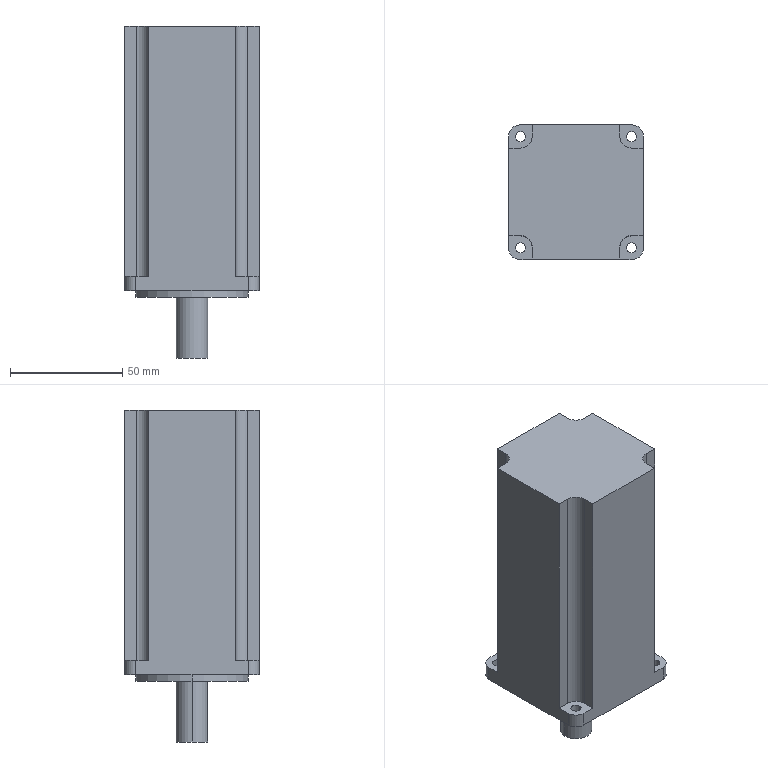Part | SolidWorks | features ICE 3, Extrusion 1 | 1 solid | 40 faces | box 60 x 60 x 148 mm | volume 387738 mm3 | cylinder 20 | plane 20 | commonest cylinder face diameters 4.5 x8 10 x4 10.503 x4 14 x2 50 x2
STEP:
#1=CARTESIAN_POINT('',(-7.,0.,-30.));
#2=VERTEX_POINT('',#1);
#3=CARTESIAN_POINT('',(7.,0.,-30.));
#4=VERTEX_POINT('',#3);
#5=CARTESIAN_POINT('',(0.,0.,-30.));
#6=DIRECTION('',(0.,0.,-1.));
#7=DIRECTION('',(-1.,0.,0.));
#8=AXIS2_PLACEMENT_3D('',#5,#6,#7);
#9=CIRCLE('',#8,7.);
#10=EDGE_CURVE('',#2,#4,#9,.T.);
#11=ORIENTED_EDGE('',*,*,#10,.F.);
#12=CARTESIAN_POINT('',(-7.,0.,-3.));
#13=VERTEX_POINT('',#12);
#14=CARTESIAN_POINT('',(-7.,0.,-30.));
#15=DIRECTION('',(0.,0.,1.));
#16=VECTOR('',#15,1000.);
#17=LINE('',#14,#16);
#18=EDGE_CURVE('',#2,#13,#17,.T.);
#19=ORIENTED_EDGE('',*,*,#18,.T.);
#20=CARTESIAN_POINT('',(7.,0.,-3.));
#21=VERTEX_POINT('',#20);
#22=CARTESIAN_POINT('',(0.,0.,-3.));
#23=DIRECTION('',(0.,0.,-1.));
#24=DIRECTION('',(-1.,0.,0.));
#25=AXIS2_PLACEMENT_3D('',#22,#23,#24);
#26=CIRCLE('',#25,7.);
#27=EDGE_CURVE('',#13,#21,#26,.T.);
#28=ORIENTED_EDGE('',*,*,#27,.T.);
#29=CARTESIAN_POINT('',(7.,0.,-30.));
#30=DIRECTION('',(0.,0.,1.));
#31=VECTOR('',#30,1000.);
#32=LINE('',#29,#31);
#33=EDGE_CURVE('',#4,#21,#32,.T.);
#34=ORIENTED_EDGE('',*,*,#33,.F.);
#35=EDGE_LOOP('',(#11,#19,#28,#34));
#36=FACE_OUTER_BOUND('',#35,.T.);
#37=CARTESIAN_POINT('',(0.,0.,-30.));
#38=DIRECTION('',(0.,0.,1.));
#39=DIRECTION('',(1.,0.,0.));
#40=AXIS2_PLACEMENT_3D('',#37,#38,#39);
#41=CYLINDRICAL_SURFACE('',#40,7.);
#42=ADVANCED_FACE('',(#36),#41,.T.);
#43=CARTESIAN_POINT('',(-25.,0.,-3.));
#44=VERTEX_POINT('',#43);
#45=CARTESIAN_POINT('',(25.,0.,-3.));
#46=VERTEX_POINT('',#45);
#47=CARTESIAN_POINT('',(0.,0.,-3.));
#48=DIRECTION('',(0.,0.,-1.));
#49=DIRECTION('',(-1.,0.,0.));
#50=AXIS2_PLACEMENT_3D('',#47,#48,#49);
#51=CIRCLE('',#50,25.);
#52=EDGE_CURVE('',#44,#46,#51,.T.);
#53=ORIENTED_EDGE('',*,*,#52,.F.);
#54=CARTESIAN_POINT('',(-25.,0.,0.));
#55=VERTEX_POINT('',#54);
#56=CARTESIAN_POINT('',(-25.,0.,-3.));
#57=DIRECTION('',(0.,0.,1.));
#58=VECTOR('',#57,1000.);
#59=LINE('',#56,#58);
#60=EDGE_CURVE('',#44,#55,#59,.T.);
#61=ORIENTED_EDGE('',*,*,#60,.T.);
#62=CARTESIAN_POINT('',(25.,0.,0.));
#63=VERTEX_POINT('',#62);
#64=CARTESIAN_POINT('',(0.,0.,0.));
#65=DIRECTION('',(0.,0.,-1.));
#66=DIRECTION('',(-1.,0.,0.));
#67=AXIS2_PLACEMENT_3D('',#64,#65,#66);
#68=CIRCLE('',#67,25.);
#69=EDGE_CURVE('',#55,#63,#68,.T.);
#70=ORIENTED_EDGE('',*,*,#69,.T.);
#71=CARTESIAN_POINT('',(25.,0.,-3.));
#72=DIRECTION('',(0.,0.,1.));
#73=VECTOR('',#72,1000.);
#74=LINE('',#71,#73);
#75=EDGE_CURVE('',#46,#63,#74,.T.);
#76=ORIENTED_EDGE('',*,*,#75,.F.);
#77=EDGE_LOOP('',(#53,#61,#70,#76));
#78=FACE_OUTER_BOUND('',#77,.T.);
#79=CARTESIAN_POINT('',(0.,0.,-3.));
#80=DIRECTION('',(0.,0.,1.));
#81=DIRECTION('',(1.,0.,0.));
#82=AXIS2_PLACEMENT_3D('',#79,#80,#81);
#83=CYLINDRICAL_SURFACE('',#82,25.);
#84=ADVANCED_FACE('',(#78),#83,.T.);
#85=CARTESIAN_POINT('',(22.499,24.749,6.5));
#86=VERTEX_POINT('',#85);
#87=CARTESIAN_POINT('',(26.999,24.749,6.5));
#88=VERTEX_POINT('',#87);
#89=CARTESIAN_POINT('',(24.749,24.749,6.5));
#90=DIRECTION('',(0.,0.,1.));
#91=DIRECTION('',(1.,0.,0.));
#92=AXIS2_PLACEMENT_3D('',#89,#90,#91);
#93=CIRCLE('',#92,2.25);
#94=EDGE_CURVE('',#86,#88,#93,.T.);
#95=ORIENTED_EDGE('',*,*,#94,.T.);
#96=CARTESIAN_POINT('',(26.999,24.749,0.));
#97=VERTEX_POINT('',#96);
#98=CARTESIAN_POINT('',(26.999,24.749,6.5));
#99=DIRECTION('',(0.,0.,-1.));
#100=VECTOR('',#99,1000.);
#101=LINE('',#98,#100);
#102=EDGE_CURVE('',#88,#97,#101,.T.);
#103=ORIENTED_EDGE('',*,*,#102,.T.);
#104=CARTESIAN_POINT('',(22.499,24.749,0.));
#105=VERTEX_POINT('',#104);
#106=CARTESIAN_POINT('',(24.749,24.749,0.));
#107=DIRECTION('',(0.,0.,1.));
#108=DIRECTION('',(1.,0.,0.));
#109=AXIS2_PLACEMENT_3D('',#106,#107,#108);
#110=CIRCLE('',#109,2.25);
#111=EDGE_CURVE('',#105,#97,#110,.T.);
#112=ORIENTED_EDGE('',*,*,#111,.F.);
#113=CARTESIAN_POINT('',(22.499,24.749,6.5));
#114=DIRECTION('',(0.,0.,-1.));
#115=VECTOR('',#114,1000.);
#116=LINE('',#113,#115);
#117=EDGE_CURVE('',#86,#105,#116,.T.);
#118=ORIENTED_EDGE('',*,*,#117,.F.);
#119=EDGE_LOOP('',(#95,#103,#112,#118));
#120=FACE_OUTER_BOUND('',#119,.T.);
#121=CARTESIAN_POINT('',(24.749,24.749,6.5));
#122=DIRECTION('',(0.,0.,-1.));
#123=DIRECTION('',(-1.,0.,0.));
#124=AXIS2_PLACEMENT_3D('',#121,#122,#123);
#125=CYLINDRICAL_SURFACE('',#124,2.25);
#126=ADVANCED_FACE('',(#120),#125,.F.);
#127=CARTESIAN_POINT('',(22.499,-24.749,6.5));
#128=VERTEX_POINT('',#127);
#129=CARTESIAN_POINT('',(26.999,-24.749,6.5));
#130=VERTEX_POINT('',#129);
#131=CARTESIAN_POINT('',(24.749,-24.749,6.5));
#132=DIRECTION('',(0.,0.,1.));
#133=DIRECTION('',(1.,0.,0.));
#134=AXIS2_PLACEMENT_3D('',#131,#132,#133);
#135=CIRCLE('',#134,2.25);
#136=EDGE_CURVE('',#128,#130,#135,.T.);
#137=ORIENTED_EDGE('',*,*,#136,.T.);
#138=CARTESIAN_POINT('',(26.999,-24.749,0.));
#139=VERTEX_POINT('',#138);
#140=CARTESIAN_POINT('',(26.999,-24.749,6.5));
#141=DIRECTION('',(0.,0.,-1.));
#142=VECTOR('',#141,1000.);
#143=LINE('',#140,#142);
#144=EDGE_CURVE('',#130,#139,#143,.T.);
#145=ORIENTED_EDGE('',*,*,#144,.T.);
#146=CARTESIAN_POINT('',(22.499,-24.749,0.));
#147=VERTEX_POINT('',#146);
#148=CARTESIAN_POINT('',(24.749,-24.749,0.));
#149=DIRECTION('',(0.,0.,1.));
#150=DIRECTION('',(1.,0.,0.));
#151=AXIS2_PLACEMENT_3D('',#148,#149,#150);
#152=CIRCLE('',#151,2.25);
#153=EDGE_CURVE('',#147,#139,#152,.T.);
#154=ORIENTED_EDGE('',*,*,#153,.F.);
#155=CARTESIAN_POINT('',(22.499,-24.749,6.5));
#156=DIRECTION('',(0.,0.,-1.));
#157=VECTOR('',#156,1000.);
#158=LINE('',#155,#157);
#159=EDGE_CURVE('',#128,#147,#158,.T.);
#160=ORIENTED_EDGE('',*,*,#159,.F.);
#161=EDGE_LOOP('',(#137,#145,#154,#160));
#162=FACE_OUTER_BOUND('',#161,.T.);
#163=CARTESIAN_POINT('',(24.749,-24.749,6.5));
#164=DIRECTION('',(0.,0.,-1.));
#165=DIRECTION('',(-1.,0.,0.));
#166=AXIS2_PLACEMENT_3D('',#163,#164,#165);
#167=CYLINDRICAL_SURFACE('',#166,2.25);
#168=ADVANCED_FACE('',(#162),#167,.F.);
#169=CARTESIAN_POINT('',(-26.999,-24.749,6.5));
#170=VERTEX_POINT('',#169);
#171=CARTESIAN_POINT('',(-22.499,-24.749,6.5));
#172=VERTEX_POINT('',#171);
#173=CARTESIAN_POINT('',(-24.749,-24.749,6.5));
#174=DIRECTION('',(0.,0.,1.));
#175=DIRECTION('',(1.,0.,0.));
#176=AXIS2_PLACEMENT_3D('',#173,#174,#175);
#177=CIRCLE('',#176,2.25);
#178=EDGE_CURVE('',#170,#172,#177,.T.);
#179=ORIENTED_EDGE('',*,*,#178,.T.);
#180=CARTESIAN_POINT('',(-22.499,-24.749,0.));
#181=VERTEX_POINT('',#180);
#182=CARTESIAN_POINT('',(-22.499,-24.749,6.5));
#183=DIRECTION('',(0.,0.,-1.));
#184=VECTOR('',#183,1000.);
#185=LINE('',#182,#184);
#186=EDGE_CURVE('',#172,#181,#185,.T.);
#187=ORIENTED_EDGE('',*,*,#186,.T.);
#188=CARTESIAN_POINT('',(-26.999,-24.749,0.));
#189=VERTEX_POINT('',#188);
#190=CARTESIAN_POINT('',(-24.749,-24.749,0.));
#191=DIRECTION('',(0.,0.,1.));
#192=DIRECTION('',(1.,0.,0.));
#193=AXIS2_PLACEMENT_3D('',#190,#191,#192);
#194=CIRCLE('',#193,2.25);
#195=EDGE_CURVE('',#189,#181,#194,.T.);
#196=ORIENTED_EDGE('',*,*,#195,.F.);
#197=CARTESIAN_POINT('',(-26.999,-24.749,6.5));
#198=DIRECTION('',(0.,0.,-1.));
#199=VECTOR('',#198,1000.);
#200=LINE('',#197,#199);
#201=EDGE_CURVE('',#170,#189,#200,.T.);
#202=ORIENTED_EDGE('',*,*,#201,.F.);
#203=EDGE_LOOP('',(#179,#187,#196,#202));
#204=FACE_OUTER_BOUND('',#203,.T.);
#205=CARTESIAN_POINT('',(-24.749,-24.749,6.5));
#206=DIRECTION('',(0.,0.,-1.));
#207=DIRECTION('',(-1.,0.,0.));
#208=AXIS2_PLACEMENT_3D('',#205,#206,#207);
#209=CYLINDRICAL_SURFACE('',#208,2.25);
#210=ADVANCED_FACE('',(#204),#209,.F.);
#211=CARTESIAN_POINT('',(-26.999,24.749,6.5));
#212=VERTEX_POINT('',#211);
#213=CARTESIAN_POINT('',(-22.499,24.749,6.5));
#214=VERTEX_POINT('',#213);
#215=CARTESIAN_POINT('',(-24.749,24.749,6.5));
#216=DIRECTION('',(0.,0.,1.));
#217=DIRECTION('',(1.,0.,0.));
#218=AXIS2_PLACEMENT_3D('',#215,#216,#217);
#219=CIRCLE('',#218,2.25);
#220=EDGE_CURVE('',#212,#214,#219,.T.);
#221=ORIENTED_EDGE('',*,*,#220,.T.);
#222=CARTESIAN_POINT('',(-22.499,24.749,0.));
#223=VERTEX_POINT('',#222);
#224=CARTESIAN_POINT('',(-22.499,24.749,6.5));
#225=DIRECTION('',(0.,0.,-1.));
#226=VECTOR('',#225,1000.);
#227=LINE('',#224,#226);
#228=EDGE_CURVE('',#214,#223,#227,.T.);
#229=ORIENTED_EDGE('',*,*,#228,.T.);
#230=CARTESIAN_POINT('',(-26.999,24.749,0.));
#231=VERTEX_POINT('',#230);
#232=CARTESIAN_POINT('',(-24.749,24.749,0.));
#233=DIRECTION('',(0.,0.,1.));
#234=DIRECTION('',(1.,0.,0.));
#235=AXIS2_PLACEMENT_3D('',#232,#233,#234);
#236=CIRCLE('',#235,2.25);
#237=EDGE_CURVE('',#231,#223,#236,.T.);
#238=ORIENTED_EDGE('',*,*,#237,.F.);
#239=CARTESIAN_POINT('',(-26.999,24.749,6.5));
#240=DIRECTION('',(0.,0.,-1.));
#241=VECTOR('',#240,1000.);
#242=LINE('',#239,#241);
#243=EDGE_CURVE('',#212,#231,#242,.T.);
#244=ORIENTED_EDGE('',*,*,#243,.F.);
#245=EDGE_LOOP('',(#221,#229,#238,#244));
#246=FACE_OUTER_BOUND('',#245,.T.);
#247=CARTESIAN_POINT('',(-24.749,24.749,6.5));
#248=DIRECTION('',(0.,0.,-1.));
#249=DIRECTION('',(-1.,0.,0.));
#250=AXIS2_PLACEMENT_3D('',#247,#248,#249);
#251=CYLINDRICAL_SURFACE('',#250,2.25);
#252=ADVANCED_FACE('',(#246),#251,.F.);
#253=CARTESIAN_POINT('',(0.,0.,-3.));
#254=DIRECTION('',(0.,0.,-1.));
#255=DIRECTION('',(-1.,0.,0.));
#256=AXIS2_PLACEMENT_3D('',#253,#254,#255);
#257=CIRCLE('',#256,25.);
#258=EDGE_CURVE('',#46,#44,#257,.T.);
#259=ORIENTED_EDGE('',*,*,#258,.T.);
#260=ORIENTED_EDGE('',*,*,#52,.T.);
#261=EDGE_LOOP('',(#259,#260));
#262=FACE_OUTER_BOUND('',#261,.T.);
#263=CARTESIAN_POINT('',(0.,0.,-3.));
#264=DIRECTION('',(0.,0.,-1.));
#265=DIRECTION('',(-1.,0.,0.));
#266=AXIS2_PLACEMENT_3D('',#263,#264,#265);
#267=CIRCLE('',#266,7.);
#268=EDGE_CURVE('',#21,#13,#267,.T.);
#269=ORIENTED_EDGE('',*,*,#268,.F.);
#270=ORIENTED_EDGE('',*,*,#27,.F.);
#271=EDGE_LOOP('',(#269,#270));
#272=FACE_BOUND('',#271,.T.);
#273=CARTESIAN_POINT('',(0.,0.,-3.));
#274=DIRECTION('',(0.,0.,-1.));
#275=DIRECTION('',(-1.,0.,0.));
#276=AXIS2_PLACEMENT_3D('',#273,#274,#275);
#277=PLANE('',#276);
#278=ADVANCED_FACE('',(#262,#272),#277,.T.);
#279=ORIENTED_EDGE('',*,*,#111,.T.);
#280=CARTESIAN_POINT('',(24.749,24.749,0.));
#281=DIRECTION('',(0.,0.,1.));
#282=DIRECTION('',(1.,0.,0.));
#283=AXIS2_PLACEMENT_3D('',#280,#281,#282);
#284=CIRCLE('',#283,2.25);
#285=EDGE_CURVE('',#97,#105,#284,.T.);
#286=ORIENTED_EDGE('',*,*,#285,.T.);
#287=EDGE_LOOP('',(#279,#286));
#288=FACE_BOUND('',#287,.T.);
#289=ORIENTED_EDGE('',*,*,#195,.T.);
#290=CARTESIAN_POINT('',(-24.749,-24.749,0.));
#291=DIRECTION('',(0.,0.,1.));
#292=DIRECTION('',(1.,0.,0.));
#293=AXIS2_PLACEMENT_3D('',#290,#291,#292);
#294=CIRCLE('',#293,2.25);
#295=EDGE_CURVE('',#181,#189,#294,.T.);
#296=ORIENTED_EDGE('',*,*,#295,.T.);
#297=EDGE_LOOP('',(#289,#296));
#298=FACE_BOUND('',#297,.T.);
#299=CARTESIAN_POINT('',(-25.,30.,0.));
#300=VERTEX_POINT('',#299);
#301=CARTESIAN_POINT('',(-30.,25.,0.));
#302=VERTEX_POINT('',#301);
#303=CARTESIAN_POINT('',(-25.,25.,0.));
#304=DIRECTION('',(0.,0.,1.));
#305=DIRECTION('',(-1.,0.,0.));
#306=AXIS2_PLACEMENT_3D('',#303,#304,#305);
#307=CIRCLE('',#306,5.);
#308=EDGE_CURVE('',#300,#302,#307,.T.);
#309=ORIENTED_EDGE('',*,*,#308,.F.);
#310=CARTESIAN_POINT('',(25.,30.,0.));
#311=VERTEX_POINT('',#310);
#312=CARTESIAN_POINT('',(-25.,30.,0.));
#313=DIRECTION('',(-1.,0.,0.));
#314=VECTOR('',#313,1000.);
#315=LINE('',#312,#314);
#316=EDGE_CURVE('',#311,#300,#315,.T.);
#317=ORIENTED_EDGE('',*,*,#316,.F.);
#318=CARTESIAN_POINT('',(30.,25.,0.));
#319=VERTEX_POINT('',#318);
#320=CARTESIAN_POINT('',(25.,25.,0.));
#321=DIRECTION('',(0.,0.,1.));
#322=DIRECTION('',(-1.,0.,0.));
#323=AXIS2_PLACEMENT_3D('',#320,#321,#322);
#324=CIRCLE('',#323,5.);
#325=EDGE_CURVE('',#319,#311,#324,.T.);
#326=ORIENTED_EDGE('',*,*,#325,.F.);
#327=CARTESIAN_POINT('',(30.,-25.,0.));
#328=VERTEX_POINT('',#327);
#329=CARTESIAN_POINT('',(30.,-25.,0.));
#330=DIRECTION('',(0.,1.,0.));
#331=VECTOR('',#330,1000.);
#332=LINE('',#329,#331);
#333=EDGE_CURVE('',#328,#319,#332,.T.);
#334=ORIENTED_EDGE('',*,*,#333,.F.);
#335=CARTESIAN_POINT('',(25.,-30.,0.));
#336=VERTEX_POINT('',#335);
#337=CARTESIAN_POINT('',(25.,-25.,0.));
#338=DIRECTION('',(0.,0.,1.));
#339=DIRECTION('',(1.,0.,0.));
#340=AXIS2_PLACEMENT_3D('',#337,#338,#339);
#341=CIRCLE('',#340,5.);
#342=EDGE_CURVE('',#336,#328,#341,.T.);
#343=ORIENTED_EDGE('',*,*,#342,.F.);
#344=CARTESIAN_POINT('',(-25.,-30.,0.));
#345=VERTEX_POINT('',#344);
#346=CARTESIAN_POINT('',(-25.,-30.,0.));
#347=DIRECTION('',(1.,0.,0.));
#348=VECTOR('',#347,1000.);
#349=LINE('',#346,#348);
#350=EDGE_CURVE('',#345,#336,#349,.T.);
#351=ORIENTED_EDGE('',*,*,#350,.F.);
#352=CARTESIAN_POINT('',(-30.,-25.,0.));
#353=VERTEX_POINT('',#352);
#354=CARTESIAN_POINT('',(-25.,-25.,0.));
#355=DIRECTION('',(0.,0.,1.));
#356=DIRECTION('',(1.,0.,0.));
#357=AXIS2_PLACEMENT_3D('',#354,#355,#356);
#358=CIRCLE('',#357,5.);
#359=EDGE_CURVE('',#353,#345,#358,.T.);
#360=ORIENTED_EDGE('',*,*,#359,.F.);
#361=CARTESIAN_POINT('',(-30.,-25.,0.));
#362=DIRECTION('',(0.,-1.,0.));
#363=VECTOR('',#362,1000.);
#364=LINE('',#361,#363);
#365=EDGE_CURVE('',#302,#353,#364,.T.);
#366=ORIENTED_EDGE('',*,*,#365,.F.);
#367=EDGE_LOOP('',(#309,#317,#326,#334,#343,#351,#360,#366));
#368=FACE_OUTER_BOUND('',#367,.T.);
#369=ORIENTED_EDGE('',*,*,#237,.T.);
#370=CARTESIAN_POINT('',(-24.749,24.749,0.));
#371=DIRECTION('',(0.,0.,1.));
#372=DIRECTION('',(1.,0.,0.));
#373=AXIS2_PLACEMENT_3D('',#370,#371,#372);
#374=CIRCLE('',#373,2.25);
#375=EDGE_CURVE('',#223,#231,#374,.T.);
#376=ORIENTED_EDGE('',*,*,#375,.T.);
#377=EDGE_LOOP('',(#369,#376));
#378=FACE_BOUND('',#377,.T.);
#379=ORIENTED_EDGE('',*,*,#153,.T.);
#380=CARTESIAN_POINT('',(24.749,-24.749,0.));
#381=DIRECTION('',(0.,0.,1.));
#382=DIRECTION('',(1.,0.,0.));
#383=AXIS2_PLACEMENT_3D('',#380,#381,#382);
#384=CIRCLE('',#383,2.25);
#385=EDGE_CURVE('',#139,#147,#384,.T.);
#386=ORIENTED_EDGE('',*,*,#385,.T.);
#387=EDGE_LOOP('',(#379,#386));
#388=FACE_BOUND('',#387,.T.);
#389=CARTESIAN_POINT('',(0.,0.,0.));
#390=DIRECTION('',(0.,0.,-1.));
#391=DIRECTION('',(-1.,0.,0.));
#392=AXIS2_PLACEMENT_3D('',#389,#390,#391);
#393=CIRCLE('',#392,25.);
#394=EDGE_CURVE('',#63,#55,#393,.T.);
#395=ORIENTED_EDGE('',*,*,#394,.F.);
#396=ORIENTED_EDGE('',*,*,#69,.F.);
#397=EDGE_LOOP('',(#395,#396));
#398=FACE_BOUND('',#397,.T.);
#399=CARTESIAN_POINT('',(-25.,25.,0.));
#400=DIRECTION('',(0.,0.,-1.));
#401=DIRECTION('',(-1.,0.,0.));
#402=AXIS2_PLACEMENT_3D('',#399,#400,#401);
#403=PLANE('',#402);
#404=ADVANCED_FACE('',(#288,#298,#368,#378,#388,#398),#403,.T.);
#405=ORIENTED_EDGE('',*,*,#94,.F.);
#406=CARTESIAN_POINT('',(24.749,24.749,6.5));
#407=DIRECTION('',(0.,0.,1.));
#408=DIRECTION('',(1.,0.,0.));
#409=AXIS2_PLACEMENT_3D('',#406,#407,#408);
#410=CIRCLE('',#409,2.25);
#411=EDGE_CURVE('',#88,#86,#410,.T.);
#412=ORIENTED_EDGE('',*,*,#411,.F.);
#413=EDGE_LOOP('',(#405,#412));
#414=FACE_BOUND('',#413,.T.);
#415=CARTESIAN_POINT('',(19.497,24.749,6.5));
#416=VERTEX_POINT('',#415);
#417=CARTESIAN_POINT('',(19.497,30.,6.5));
#418=VERTEX_POINT('',#417);
#419=CARTESIAN_POINT('',(19.497,24.749,6.5));
#420=DIRECTION('',(0.,1.,0.));
#421=VECTOR('',#420,1000.);
#422=LINE('',#419,#421);
#423=EDGE_CURVE('',#416,#418,#422,.T.);
#424=ORIENTED_EDGE('',*,*,#423,.F.);
#425=CARTESIAN_POINT('',(24.749,19.497,6.5));
#426=VERTEX_POINT('',#425);
#427=CARTESIAN_POINT('',(24.749,24.749,6.5));
#428=DIRECTION('',(0.,0.,-1.));
#429=DIRECTION('',(1.,0.,0.));
#430=AXIS2_PLACEMENT_3D('',#427,#428,#429);
#431=CIRCLE('',#430,5.251);
#432=EDGE_CURVE('',#426,#416,#431,.T.);
#433=ORIENTED_EDGE('',*,*,#432,.F.);
#434=CARTESIAN_POINT('',(30.,19.497,6.5));
#435=VERTEX_POINT('',#434);
#436=CARTESIAN_POINT('',(24.749,19.497,6.5));
#437=DIRECTION('',(-1.,0.,0.));
#438=VECTOR('',#437,1000.);
#439=LINE('',#436,#438);
#440=EDGE_CURVE('',#435,#426,#439,.T.);
#441=ORIENTED_EDGE('',*,*,#440,.F.);
#442=CARTESIAN_POINT('',(30.,25.,6.5));
#443=VERTEX_POINT('',#442);
#444=CARTESIAN_POINT('',(30.,-25.,6.5));
#445=DIRECTION('',(0.,1.,0.));
#446=VECTOR('',#445,1000.);
#447=LINE('',#444,#446);
#448=EDGE_CURVE('',#435,#443,#447,.T.);
#449=ORIENTED_EDGE('',*,*,#448,.T.);
#450=CARTESIAN_POINT('',(25.,30.,6.5));
#451=VERTEX_POINT('',#450);
#452=CARTESIAN_POINT('',(25.,25.,6.5));
#453=DIRECTION('',(0.,0.,1.));
#454=DIRECTION('',(-1.,0.,0.));
#455=AXIS2_PLACEMENT_3D('',#452,#453,#454);
#456=CIRCLE('',#455,5.);
#457=EDGE_CURVE('',#443,#451,#456,.T.);
#458=ORIENTED_EDGE('',*,*,#457,.T.);
#459=CARTESIAN_POINT('',(-25.,30.,6.5));
#460=DIRECTION('',(-1.,0.,0.));
#461=VECTOR('',#460,1000.);
#462=LINE('',#459,#461);
#463=EDGE_CURVE('',#451,#418,#462,.T.);
#464=ORIENTED_EDGE('',*,*,#463,.T.);
#465=EDGE_LOOP('',(#424,#433,#441,#449,#458,#464));
#466=FACE_OUTER_BOUND('',#465,.T.);
#467=CARTESIAN_POINT('',(-25.,25.,6.5));
#468=DIRECTION('',(0.,0.,-1.));
#469=DIRECTION('',(-1.,0.,0.));
#470=AXIS2_PLACEMENT_3D('',#467,#468,#469);
#471=PLANE('',#470);
#472=ADVANCED_FACE('',(#414,#466),#471,.F.);
#473=ORIENTED_EDGE('',*,*,#136,.F.);
#474=CARTESIAN_POINT('',(24.749,-24.749,6.5));
#475=DIRECTION('',(0.,0.,1.));
#476=DIRECTION('',(1.,0.,0.));
#477=AXIS2_PLACEMENT_3D('',#474,#475,#476);
#478=CIRCLE('',#477,2.25);
#479=EDGE_CURVE('',#130,#128,#478,.T.);
#480=ORIENTED_EDGE('',*,*,#479,.F.);
#481=EDGE_LOOP('',(#473,#480));
#482=FACE_BOUND('',#481,.T.);
#483=CARTESIAN_POINT('',(24.749,-19.497,6.5));
#484=VERTEX_POINT('',#483);
#485=CARTESIAN_POINT('',(30.,-19.497,6.5));
#486=VERTEX_POINT('',#485);
#487=CARTESIAN_POINT('',(24.749,-19.497,6.5));
#488=DIRECTION('',(1.,0.,0.));
#489=VECTOR('',#488,1000.);
#490=LINE('',#487,#489);
#491=EDGE_CURVE('',#484,#486,#490,.T.);
#492=ORIENTED_EDGE('',*,*,#491,.F.);
#493=CARTESIAN_POINT('',(19.497,-24.749,6.5));
#494=VERTEX_POINT('',#493);
#495=CARTESIAN_POINT('',(24.749,-24.749,6.5));
#496=DIRECTION('',(0.,0.,-1.));
#497=DIRECTION('',(1.,0.,0.));
#498=AXIS2_PLACEMENT_3D('',#495,#496,#497);
#499=CIRCLE('',#498,5.251);
#500=EDGE_CURVE('',#494,#484,#499,.T.);
#501=ORIENTED_EDGE('',*,*,#500,.F.);
#502=CARTESIAN_POINT('',(19.497,-30.,6.5));
#503=VERTEX_POINT('',#502);
#504=CARTESIAN_POINT('',(19.497,-24.749,6.5));
#505=DIRECTION('',(0.,1.,0.));
#506=VECTOR('',#505,1000.);
#507=LINE('',#504,#506);
#508=EDGE_CURVE('',#503,#494,#507,.T.);
#509=ORIENTED_EDGE('',*,*,#508,.F.);
#510=CARTESIAN_POINT('',(25.,-30.,6.5));
#511=VERTEX_POINT('',#510);
#512=CARTESIAN_POINT('',(-25.,-30.,6.5));
#513=DIRECTION('',(1.,0.,0.));
#514=VECTOR('',#513,1000.);
#515=LINE('',#512,#514);
#516=EDGE_CURVE('',#503,#511,#515,.T.);
#517=ORIENTED_EDGE('',*,*,#516,.T.);
#518=CARTESIAN_POINT('',(30.,-25.,6.5));
#519=VERTEX_POINT('',#518);
#520=CARTESIAN_POINT('',(25.,-25.,6.5));
#521=DIRECTION('',(0.,0.,1.));
#522=DIRECTION('',(1.,0.,0.));
#523=AXIS2_PLACEMENT_3D('',#520,#521,#522);
#524=CIRCLE('',#523,5.);
#525=EDGE_CURVE('',#511,#519,#524,.T.);
#526=ORIENTED_EDGE('',*,*,#525,.T.);
#527=CARTESIAN_POINT('',(30.,-25.,6.5));
#528=DIRECTION('',(0.,1.,0.));
#529=VECTOR('',#528,1000.);
#530=LINE('',#527,#529);
#531=EDGE_CURVE('',#519,#486,#530,.T.);
#532=ORIENTED_EDGE('',*,*,#531,.T.);
#533=EDGE_LOOP('',(#492,#501,#509,#517,#526,#532));
#534=FACE_OUTER_BOUND('',#533,.T.);
#535=CARTESIAN_POINT('',(-25.,25.,6.5));
#536=DIRECTION('',(0.,0.,-1.));
#537=DIRECTION('',(-1.,0.,0.));
#538=AXIS2_PLACEMENT_3D('',#535,#536,#537);
#539=PLANE('',#538);
#540=ADVANCED_FACE('',(#482,#534),#539,.F.);
#541=ORIENTED_EDGE('',*,*,#178,.F.);
#542=CARTESIAN_POINT('',(-24.749,-24.749,6.5));
#543=DIRECTION('',(0.,0.,1.));
#544=DIRECTION('',(1.,0.,0.));
#545=AXIS2_PLACEMENT_3D('',#542,#543,#544);
#546=CIRCLE('',#545,2.25);
#547=EDGE_CURVE('',#172,#170,#546,.T.);
#548=ORIENTED_EDGE('',*,*,#547,.F.);
#549=EDGE_LOOP('',(#541,#548));
#550=FACE_BOUND('',#549,.T.);
#551=CARTESIAN_POINT('',(-19.497,-24.749,6.5));
#552=VERTEX_POINT('',#551);
#553=CARTESIAN_POINT('',(-19.497,-30.,6.5));
#554=VERTEX_POINT('',#553);
#555=CARTESIAN_POINT('',(-19.497,-24.749,6.5));
#556=DIRECTION('',(0.,-1.,0.));
#557=VECTOR('',#556,1000.);
#558=LINE('',#555,#557);
#559=EDGE_CURVE('',#552,#554,#558,.T.);
#560=ORIENTED_EDGE('',*,*,#559,.F.);
#561=CARTESIAN_POINT('',(-24.749,-19.497,6.5));
#562=VERTEX_POINT('',#561);
#563=CARTESIAN_POINT('',(-24.749,-24.749,6.5));
#564=DIRECTION('',(0.,0.,-1.));
#565=DIRECTION('',(1.,0.,0.));
#566=AXIS2_PLACEMENT_3D('',#563,#564,#565);
#567=CIRCLE('',#566,5.251);
#568=EDGE_CURVE('',#562,#552,#567,.T.);
#569=ORIENTED_EDGE('',*,*,#568,.F.);
#570=CARTESIAN_POINT('',(-30.,-19.497,6.5));
#571=VERTEX_POINT('',#570);
#572=CARTESIAN_POINT('',(-24.749,-19.497,6.5));
#573=DIRECTION('',(1.,0.,0.));
#574=VECTOR('',#573,1000.);
#575=LINE('',#572,#574);
#576=EDGE_CURVE('',#571,#562,#575,.T.);
#577=ORIENTED_EDGE('',*,*,#576,.F.);
#578=CARTESIAN_POINT('',(-30.,-25.,6.5));
#579=VERTEX_POINT('',#578);
#580=CARTESIAN_POINT('',(-30.,-25.,6.5));
#581=DIRECTION('',(0.,-1.,0.));
#582=VECTOR('',#581,1000.);
#583=LINE('',#580,#582);
#584=EDGE_CURVE('',#571,#579,#583,.T.);
#585=ORIENTED_EDGE('',*,*,#584,.T.);
#586=CARTESIAN_POINT('',(-25.,-30.,6.5));
#587=VERTEX_POINT('',#586);
#588=CARTESIAN_POINT('',(-25.,-25.,6.5));
#589=DIRECTION('',(0.,0.,1.));
#590=DIRECTION('',(1.,0.,0.));
#591=AXIS2_PLACEMENT_3D('',#588,#589,#590);
#592=CIRCLE('',#591,5.);
#593=EDGE_CURVE('',#579,#587,#592,.T.);
#594=ORIENTED_EDGE('',*,*,#593,.T.);
#595=CARTESIAN_POINT('',(-25.,-30.,6.5));
#596=DIRECTION('',(1.,0.,0.));
#597=VECTOR('',#596,1000.);
#598=LINE('',#595,#597);
#599=EDGE_CURVE('',#587,#554,#598,.T.);
#600=ORIENTED_EDGE('',*,*,#599,.T.);
#601=EDGE_LOOP('',(#560,#569,#577,#585,#594,#600));
#602=FACE_OUTER_BOUND('',#601,.T.);
#603=CARTESIAN_POINT('',(-25.,25.,6.5));
#604=DIRECTION('',(0.,0.,-1.));
#605=DIRECTION('',(-1.,0.,0.));
#606=AXIS2_PLACEMENT_3D('',#603,#604,#605);
#607=PLANE('',#606);
#608=ADVANCED_FACE('',(#550,#602),#607,.F.);
#609=ORIENTED_EDGE('',*,*,#220,.F.);
#610=CARTESIAN_POINT('',(-24.749,24.749,6.5));
#611=DIRECTION('',(0.,0.,1.));
#612=DIRECTION('',(1.,0.,0.));
#613=AXIS2_PLACEMENT_3D('',#610,#611,#612);
#614=CIRCLE('',#613,2.25);
#615=EDGE_CURVE('',#214,#212,#614,.T.);
#616=ORIENTED_EDGE('',*,*,#615,.F.);
#617=EDGE_LOOP('',(#609,#616));
#618=FACE_BOUND('',#617,.T.);
#619=CARTESIAN_POINT('',(-19.497,30.,6.5));
#620=VERTEX_POINT('',#619);
#621=CARTESIAN_POINT('',(-19.497,24.749,6.5));
#622=VERTEX_POINT('',#621);
#623=CARTESIAN_POINT('',(-19.497,24.749,6.5));
#624=DIRECTION('',(0.,-1.,0.));
#625=VECTOR('',#624,1000.);
#626=LINE('',#623,#625);
#627=EDGE_CURVE('',#620,#622,#626,.T.);
#628=ORIENTED_EDGE('',*,*,#627,.F.);
#629=CARTESIAN_POINT('',(-25.,30.,6.5));
#630=VERTEX_POINT('',#629);
#631=CARTESIAN_POINT('',(-25.,30.,6.5));
#632=DIRECTION('',(-1.,0.,0.));
#633=VECTOR('',#632,1000.);
#634=LINE('',#631,#633);
#635=EDGE_CURVE('',#620,#630,#634,.T.);
#636=ORIENTED_EDGE('',*,*,#635,.T.);
#637=CARTESIAN_POINT('',(-30.,25.,6.5));
#638=VERTEX_POINT('',#637);
#639=CARTESIAN_POINT('',(-25.,25.,6.5));
#640=DIRECTION('',(0.,0.,1.));
#641=DIRECTION('',(-1.,0.,0.));
#642=AXIS2_PLACEMENT_3D('',#639,#640,#641);
#643=CIRCLE('',#642,5.);
#644=EDGE_CURVE('',#630,#638,#643,.T.);
#645=ORIENTED_EDGE('',*,*,#644,.T.);
#646=CARTESIAN_POINT('',(-30.,19.497,6.5));
#647=VERTEX_POINT('',#646);
#648=CARTESIAN_POINT('',(-30.,-25.,6.5));
#649=DIRECTION('',(0.,-1.,0.));
#650=VECTOR('',#649,1000.);
#651=LINE('',#648,#650);
#652=EDGE_CURVE('',#638,#647,#651,.T.);
#653=ORIENTED_EDGE('',*,*,#652,.T.);
#654=CARTESIAN_POINT('',(-24.749,19.497,6.5));
#655=VERTEX_POINT('',#654);
#656=CARTESIAN_POINT('',(-24.749,19.497,6.5));
#657=DIRECTION('',(-1.,0.,0.));
#658=VECTOR('',#657,1000.);
#659=LINE('',#656,#658);
#660=EDGE_CURVE('',#655,#647,#659,.T.);
#661=ORIENTED_EDGE('',*,*,#660,.F.);
#662=CARTESIAN_POINT('',(-24.749,24.749,6.5));
#663=DIRECTION('',(0.,0.,-1.));
#664=DIRECTION('',(1.,0.,0.));
#665=AXIS2_PLACEMENT_3D('',#662,#663,#664);
#666=CIRCLE('',#665,5.251);
#667=EDGE_CURVE('',#622,#655,#666,.T.);
#668=ORIENTED_EDGE('',*,*,#667,.F.);
#669=EDGE_LOOP('',(#628,#636,#645,#653,#661,#668));
#670=FACE_OUTER_BOUND('',#669,.T.);
#671=CARTESIAN_POINT('',(-25.,25.,6.5));
#672=DIRECTION('',(0.,0.,-1.));
#673=DIRECTION('',(-1.,0.,0.));
#674=AXIS2_PLACEMENT_3D('',#671,#672,#673);
#675=PLANE('',#674);
#676=ADVANCED_FACE('',(#618,#670),#675,.F.);
#677=ORIENTED_EDGE('',*,*,#308,.T.);
#678=CARTESIAN_POINT('',(-30.,25.,6.5));
#679=DIRECTION('',(0.,0.,-1.));
#680=VECTOR('',#679,1000.);
#681=LINE('',#678,#680);
#682=EDGE_CURVE('',#638,#302,#681,.T.);
#683=ORIENTED_EDGE('',*,*,#682,.F.);
#684=ORIENTED_EDGE('',*,*,#644,.F.);
#685=CARTESIAN_POINT('',(-25.,30.,6.5));
#686=DIRECTION('',(0.,0.,-1.));
#687=VECTOR('',#686,1000.);
#688=LINE('',#685,#687);
#689=EDGE_CURVE('',#630,#300,#688,.T.);
#690=ORIENTED_EDGE('',*,*,#689,.T.);
#691=EDGE_LOOP('',(#677,#683,#684,#690));
#692=FACE_OUTER_BOUND('',#691,.T.);
#693=CARTESIAN_POINT('',(-25.,25.,6.5));
#694=DIRECTION('',(0.,0.,-1.));
#695=DIRECTION('',(-1.,0.,0.));
#696=AXIS2_PLACEMENT_3D('',#693,#694,#695);
#697=CYLINDRICAL_SURFACE('',#696,5.);
#698=ADVANCED_FACE('',(#692),#697,.T.);
#699=ORIENTED_EDGE('',*,*,#365,.T.);
#700=CARTESIAN_POINT('',(-30.,-25.,6.5));
#701=DIRECTION('',(0.,0.,-1.));
#702=VECTOR('',#701,1000.);
#703=LINE('',#700,#702);
#704=EDGE_CURVE('',#579,#353,#703,.T.);
#705=ORIENTED_EDGE('',*,*,#704,.F.);
#706=ORIENTED_EDGE('',*,*,#584,.F.);
#707=CARTESIAN_POINT('',(-30.,-19.497,118.));
#708=VERTEX_POINT('',#707);
#709=CARTESIAN_POINT('',(-30.,-19.497,118.));
#710=DIRECTION('',(0.,0.,-1.));
#711=VECTOR('',#710,1000.);
#712=LINE('',#709,#711);
#713=EDGE_CURVE('',#708,#571,#712,.T.);
#714=ORIENTED_EDGE('',*,*,#713,.F.);
#715=CARTESIAN_POINT('',(-30.,19.497,118.));
#716=VERTEX_POINT('',#715);
#717=CARTESIAN_POINT('',(-30.,19.497,118.));
#718=DIRECTION('',(0.,-1.,0.));
#719=VECTOR('',#718,1000.);
#720=LINE('',#717,#719);
#721=EDGE_CURVE('',#716,#708,#720,.T.);
#722=ORIENTED_EDGE('',*,*,#721,.F.);
#723=CARTESIAN_POINT('',(-30.,19.497,118.));
#724=DIRECTION('',(0.,0.,-1.));
#725=VECTOR('',#724,1000.);
#726=LINE('',#723,#725);
#727=EDGE_CURVE('',#716,#647,#726,.T.);
#728=ORIENTED_EDGE('',*,*,#727,.T.);
#729=ORIENTED_EDGE('',*,*,#652,.F.);
#730=ORIENTED_EDGE('',*,*,#682,.T.);
#731=EDGE_LOOP('',(#699,#705,#706,#714,#722,#728,#729,#730));
#732=FACE_OUTER_BOUND('',#731,.T.);
#733=CARTESIAN_POINT('',(-30.,-25.,6.5));
#734=DIRECTION('',(1.,0.,0.));
#735=DIRECTION('',(0.,1.,0.));
#736=AXIS2_PLACEMENT_3D('',#733,#734,#735);
#737=PLANE('',#736);
#738=ADVANCED_FACE('',(#732),#737,.F.);
#739=ORIENTED_EDGE('',*,*,#359,.T.);
#740=CARTESIAN_POINT('',(-25.,-30.,6.5));
#741=DIRECTION('',(0.,0.,-1.));
#742=VECTOR('',#741,1000.);
#743=LINE('',#740,#742);
#744=EDGE_CURVE('',#587,#345,#743,.T.);
#745=ORIENTED_EDGE('',*,*,#744,.F.);
#746=ORIENTED_EDGE('',*,*,#593,.F.);
#747=ORIENTED_EDGE('',*,*,#704,.T.);
#748=EDGE_LOOP('',(#739,#745,#746,#747));
#749=FACE_OUTER_BOUND('',#748,.T.);
#750=CARTESIAN_POINT('',(-25.,-25.,6.5));
#751=DIRECTION('',(0.,0.,-1.));
#752=DIRECTION('',(-1.,0.,0.));
#753=AXIS2_PLACEMENT_3D('',#750,#751,#752);
#754=CYLINDRICAL_SURFACE('',#753,5.);
#755=ADVANCED_FACE('',(#749),#754,.T.);
#756=ORIENTED_EDGE('',*,*,#350,.T.);
#757=CARTESIAN_POINT('',(25.,-30.,6.5));
#758=DIRECTION('',(0.,0.,-1.));
#759=VECTOR('',#758,1000.);
#760=LINE('',#757,#759);
#761=EDGE_CURVE('',#511,#336,#760,.T.);
#762=ORIENTED_EDGE('',*,*,#761,.F.);
#763=ORIENTED_EDGE('',*,*,#516,.F.);
#764=CARTESIAN_POINT('',(19.497,-30.,118.));
#765=VERTEX_POINT('',#764);
#766=CARTESIAN_POINT('',(19.497,-30.,118.));
#767=DIRECTION('',(0.,0.,-1.));
#768=VECTOR('',#767,1000.);
#769=LINE('',#766,#768);
#770=EDGE_CURVE('',#765,#503,#769,.T.);
#771=ORIENTED_EDGE('',*,*,#770,.F.);
#772=CARTESIAN_POINT('',(-19.497,-30.,118.));
#773=VERTEX_POINT('',#772);
#774=CARTESIAN_POINT('',(-19.497,-30.,118.));
#775=DIRECTION('',(1.,0.,0.));
#776=VECTOR('',#775,1000.);
#777=LINE('',#774,#776);
#778=EDGE_CURVE('',#773,#765,#777,.T.);
#779=ORIENTED_EDGE('',*,*,#778,.F.);
#780=CARTESIAN_POINT('',(-19.497,-30.,118.));
#781=DIRECTION('',(0.,0.,-1.));
#782=VECTOR('',#781,1000.);
#783=LINE('',#780,#782);
#784=EDGE_CURVE('',#773,#554,#783,.T.);
#785=ORIENTED_EDGE('',*,*,#784,.T.);
#786=ORIENTED_EDGE('',*,*,#599,.F.);
#787=ORIENTED_EDGE('',*,*,#744,.T.);
#788=EDGE_LOOP('',(#756,#762,#763,#771,#779,#785,#786,#787));
#789=FACE_OUTER_BOUND('',#788,.T.);
#790=CARTESIAN_POINT('',(-25.,-30.,6.5));
#791=DIRECTION('',(0.,1.,0.));
#792=DIRECTION('',(0.,0.,1.));
#793=AXIS2_PLACEMENT_3D('',#790,#791,#792);
#794=PLANE('',#793);
#795=ADVANCED_FACE('',(#789),#794,.F.);
#796=ORIENTED_EDGE('',*,*,#342,.T.);
#797=CARTESIAN_POINT('',(30.,-25.,6.5));
#798=DIRECTION('',(0.,0.,-1.));
#799=VECTOR('',#798,1000.);
#800=LINE('',#797,#799);
#801=EDGE_CURVE('',#519,#328,#800,.T.);
#802=ORIENTED_EDGE('',*,*,#801,.F.);
#803=ORIENTED_EDGE('',*,*,#525,.F.);
#804=ORIENTED_EDGE('',*,*,#761,.T.);
#805=EDGE_LOOP('',(#796,#802,#803,#804));
#806=FACE_OUTER_BOUND('',#805,.T.);
#807=CARTESIAN_POINT('',(25.,-25.,6.5));
#808=DIRECTION('',(0.,0.,-1.));
#809=DIRECTION('',(-1.,0.,0.));
#810=AXIS2_PLACEMENT_3D('',#807,#808,#809);
#811=CYLINDRICAL_SURFACE('',#810,5.);
#812=ADVANCED_FACE('',(#806),#811,.T.);
#813=ORIENTED_EDGE('',*,*,#333,.T.);
#814=CARTESIAN_POINT('',(30.,25.,6.5));
#815=DIRECTION('',(0.,0.,-1.));
#816=VECTOR('',#815,1000.);
#817=LINE('',#814,#816);
#818=EDGE_CURVE('',#443,#319,#817,.T.);
#819=ORIENTED_EDGE('',*,*,#818,.F.);
#820=ORIENTED_EDGE('',*,*,#448,.F.);
#821=CARTESIAN_POINT('',(30.,19.497,118.));
#822=VERTEX_POINT('',#821);
#823=CARTESIAN_POINT('',(30.,19.497,118.));
#824=DIRECTION('',(0.,0.,-1.));
#825=VECTOR('',#824,1000.);
#826=LINE('',#823,#825);
#827=EDGE_CURVE('',#822,#435,#826,.T.);
#828=ORIENTED_EDGE('',*,*,#827,.F.);
#829=CARTESIAN_POINT('',(30.,-19.497,118.));
#830=VERTEX_POINT('',#829);
#831=CARTESIAN_POINT('',(30.,19.497,118.));
#832=DIRECTION('',(0.,1.,0.));
#833=VECTOR('',#832,1000.);
#834=LINE('',#831,#833);
#835=EDGE_CURVE('',#830,#822,#834,.T.);
#836=ORIENTED_EDGE('',*,*,#835,.F.);
#837=CARTESIAN_POINT('',(30.,-19.497,118.));
#838=DIRECTION('',(0.,0.,-1.));
#839=VECTOR('',#838,1000.);
#840=LINE('',#837,#839);
#841=EDGE_CURVE('',#830,#486,#840,.T.);
#842=ORIENTED_EDGE('',*,*,#841,.T.);
#843=ORIENTED_EDGE('',*,*,#531,.F.);
#844=ORIENTED_EDGE('',*,*,#801,.T.);
#845=EDGE_LOOP('',(#813,#819,#820,#828,#836,#842,#843,#844));
#846=FACE_OUTER_BOUND('',#845,.T.);
#847=CARTESIAN_POINT('',(30.,-25.,6.5));
#848=DIRECTION('',(-1.,0.,0.));
#849=DIRECTION('',(0.,0.,1.));
#850=AXIS2_PLACEMENT_3D('',#847,#848,#849);
#851=PLANE('',#850);
#852=ADVANCED_FACE('',(#846),#851,.F.);
#853=ORIENTED_EDGE('',*,*,#325,.T.);
#854=CARTESIAN_POINT('',(25.,30.,6.5));
#855=DIRECTION('',(0.,0.,-1.));
#856=VECTOR('',#855,1000.);
#857=LINE('',#854,#856);
#858=EDGE_CURVE('',#451,#311,#857,.T.);
#859=ORIENTED_EDGE('',*,*,#858,.F.);
#860=ORIENTED_EDGE('',*,*,#457,.F.);
#861=ORIENTED_EDGE('',*,*,#818,.T.);
#862=EDGE_LOOP('',(#853,#859,#860,#861));
#863=FACE_OUTER_BOUND('',#862,.T.);
#864=CARTESIAN_POINT('',(25.,25.,6.5));
#865=DIRECTION('',(0.,0.,-1.));
#866=DIRECTION('',(-1.,0.,0.));
#867=AXIS2_PLACEMENT_3D('',#864,#865,#866);
#868=CYLINDRICAL_SURFACE('',#867,5.);
#869=ADVANCED_FACE('',(#863),#868,.T.);
#870=ORIENTED_EDGE('',*,*,#316,.T.);
#871=ORIENTED_EDGE('',*,*,#689,.F.);
#872=ORIENTED_EDGE('',*,*,#635,.F.);
#873=CARTESIAN_POINT('',(-19.497,30.,118.));
#874=VERTEX_POINT('',#873);
#875=CARTESIAN_POINT('',(-19.497,30.,118.));
#876=DIRECTION('',(0.,0.,-1.));
#877=VECTOR('',#876,1000.);
#878=LINE('',#875,#877);
#879=EDGE_CURVE('',#874,#620,#878,.T.);
#880=ORIENTED_EDGE('',*,*,#879,.F.);
#881=CARTESIAN_POINT('',(19.497,30.,118.));
#882=VERTEX_POINT('',#881);
#883=CARTESIAN_POINT('',(-19.497,30.,118.));
#884=DIRECTION('',(-1.,0.,0.));
#885=VECTOR('',#884,1000.);
#886=LINE('',#883,#885);
#887=EDGE_CURVE('',#882,#874,#886,.T.);
#888=ORIENTED_EDGE('',*,*,#887,.F.);
#889=CARTESIAN_POINT('',(19.497,30.,118.));
#890=DIRECTION('',(0.,0.,-1.));
#891=VECTOR('',#890,1000.);
#892=LINE('',#889,#891);
#893=EDGE_CURVE('',#882,#418,#892,.T.);
#894=ORIENTED_EDGE('',*,*,#893,.T.);
#895=ORIENTED_EDGE('',*,*,#463,.F.);
#896=ORIENTED_EDGE('',*,*,#858,.T.);
#897=EDGE_LOOP('',(#870,#871,#872,#880,#888,#894,#895,#896));
#898=FACE_OUTER_BOUND('',#897,.T.);
#899=CARTESIAN_POINT('',(-25.,30.,6.5));
#900=DIRECTION('',(0.,-1.,0.));
#901=DIRECTION('',(1.,0.,0.));
#902=AXIS2_PLACEMENT_3D('',#899,#900,#901);
#903=PLANE('',#902);
#904=ADVANCED_FACE('',(#898),#903,.F.);
#905=ORIENTED_EDGE('',*,*,#228,.F.);
#906=ORIENTED_EDGE('',*,*,#615,.T.);
#907=ORIENTED_EDGE('',*,*,#243,.T.);
#908=ORIENTED_EDGE('',*,*,#375,.F.);
#909=EDGE_LOOP('',(#905,#906,#907,#908));
#910=FACE_OUTER_BOUND('',#909,.T.);
#911=CARTESIAN_POINT('',(-24.749,24.749,6.5));
#912=DIRECTION('',(0.,0.,-1.));
#913=DIRECTION('',(-1.,0.,0.));
#914=AXIS2_PLACEMENT_3D('',#911,#912,#913);
#915=CYLINDRICAL_SURFACE('',#914,2.25);
#916=ADVANCED_FACE('',(#910),#915,.F.);
#917=ORIENTED_EDGE('',*,*,#186,.F.);
#918=ORIENTED_EDGE('',*,*,#547,.T.);
#919=ORIENTED_EDGE('',*,*,#201,.T.);
#920=ORIENTED_EDGE('',*,*,#295,.F.);
#921=EDGE_LOOP('',(#917,#918,#919,#920));
#922=FACE_OUTER_BOUND('',#921,.T.);
#923=CARTESIAN_POINT('',(-24.749,-24.749,6.5));
#924=DIRECTION('',(0.,0.,-1.));
#925=DIRECTION('',(-1.,0.,0.));
#926=AXIS2_PLACEMENT_3D('',#923,#924,#925);
#927=CYLINDRICAL_SURFACE('',#926,2.25);
#928=ADVANCED_FACE('',(#922),#927,.F.);
#929=ORIENTED_EDGE('',*,*,#144,.F.);
#930=ORIENTED_EDGE('',*,*,#479,.T.);
#931=ORIENTED_EDGE('',*,*,#159,.T.);
#932=ORIENTED_EDGE('',*,*,#385,.F.);
#933=EDGE_LOOP('',(#929,#930,#931,#932));
#934=FACE_OUTER_BOUND('',#933,.T.);
#935=CARTESIAN_POINT('',(24.749,-24.749,6.5));
#936=DIRECTION('',(0.,0.,-1.));
#937=DIRECTION('',(-1.,0.,0.));
#938=AXIS2_PLACEMENT_3D('',#935,#936,#937);
#939=CYLINDRICAL_SURFACE('',#938,2.25);
#940=ADVANCED_FACE('',(#934),#939,.F.);
#941=ORIENTED_EDGE('',*,*,#102,.F.);
#942=ORIENTED_EDGE('',*,*,#411,.T.);
#943=ORIENTED_EDGE('',*,*,#117,.T.);
#944=ORIENTED_EDGE('',*,*,#285,.F.);
#945=EDGE_LOOP('',(#941,#942,#943,#944));
#946=FACE_OUTER_BOUND('',#945,.T.);
#947=CARTESIAN_POINT('',(24.749,24.749,6.5));
#948=DIRECTION('',(0.,0.,-1.));
#949=DIRECTION('',(-1.,0.,0.));
#950=AXIS2_PLACEMENT_3D('',#947,#948,#949);
#951=CYLINDRICAL_SURFACE('',#950,2.25);
#952=ADVANCED_FACE('',(#946),#951,.F.);
#953=ORIENTED_EDGE('',*,*,#667,.T.);
#954=CARTESIAN_POINT('',(-24.749,19.497,118.));
#955=VERTEX_POINT('',#954);
#956=CARTESIAN_POINT('',(-24.749,19.497,118.));
#957=DIRECTION('',(0.,0.,-1.));
#958=VECTOR('',#957,1000.);
#959=LINE('',#956,#958);
#960=EDGE_CURVE('',#955,#655,#959,.T.);
#961=ORIENTED_EDGE('',*,*,#960,.F.);
#962=CARTESIAN_POINT('',(-19.497,24.749,118.));
#963=VERTEX_POINT('',#962);
#964=CARTESIAN_POINT('',(-24.749,24.749,118.));
#965=DIRECTION('',(0.,0.,-1.));
#966=DIRECTION('',(1.,0.,0.));
#967=AXIS2_PLACEMENT_3D('',#964,#965,#966);
#968=CIRCLE('',#967,5.251);
#969=EDGE_CURVE('',#963,#955,#968,.T.);
#970=ORIENTED_EDGE('',*,*,#969,.F.);
#971=CARTESIAN_POINT('',(-19.497,24.749,118.));
#972=DIRECTION('',(0.,0.,-1.));
#973=VECTOR('',#972,1000.);
#974=LINE('',#971,#973);
#975=EDGE_CURVE('',#963,#622,#974,.T.);
#976=ORIENTED_EDGE('',*,*,#975,.T.);
#977=EDGE_LOOP('',(#953,#961,#970,#976));
#978=FACE_OUTER_BOUND('',#977,.T.);
#979=CARTESIAN_POINT('',(-24.749,24.749,118.));
#980=DIRECTION('',(0.,0.,-1.));
#981=DIRECTION('',(-1.,0.,0.));
#982=AXIS2_PLACEMENT_3D('',#979,#980,#981);
#983=CYLINDRICAL_SURFACE('',#982,5.251);
#984=ADVANCED_FACE('',(#978),#983,.F.);
#985=ORIENTED_EDGE('',*,*,#660,.T.);
#986=ORIENTED_EDGE('',*,*,#727,.F.);
#987=CARTESIAN_POINT('',(-24.749,19.497,118.));
#988=DIRECTION('',(-1.,0.,0.));
#989=VECTOR('',#988,1000.);
#990=LINE('',#987,#989);
#991=EDGE_CURVE('',#955,#716,#990,.T.);
#992=ORIENTED_EDGE('',*,*,#991,.F.);
#993=ORIENTED_EDGE('',*,*,#960,.T.);
#994=EDGE_LOOP('',(#985,#986,#992,#993));
#995=FACE_OUTER_BOUND('',#994,.T.);
#996=CARTESIAN_POINT('',(-24.749,19.497,118.));
#997=DIRECTION('',(0.,-1.,0.));
#998=DIRECTION('',(0.,0.,-1.));
#999=AXIS2_PLACEMENT_3D('',#996,#997,#998);
#1000=PLANE('',#999);
#1001=ADVANCED_FACE('',(#995),#1000,.F.);
#1002=ORIENTED_EDGE('',*,*,#576,.T.);
#1003=CARTESIAN_POINT('',(-24.749,-19.497,118.));
#1004=VERTEX_POINT('',#1003);
#1005=CARTESIAN_POINT('',(-24.749,-19.497,118.));
#1006=DIRECTION('',(0.,0.,-1.));
#1007=VECTOR('',#1006,1000.);
#1008=LINE('',#1005,#1007);
#1009=EDGE_CURVE('',#1004,#562,#1008,.T.);
#1010=ORIENTED_EDGE('',*,*,#1009,.F.);
#1011=CARTESIAN_POINT('',(-24.749,-19.497,118.));
#1012=DIRECTION('',(1.,0.,0.));
#1013=VECTOR('',#1012,1000.);
#1014=LINE('',#1011,#1013);
#1015=EDGE_CURVE('',#708,#1004,#1014,.T.);
#1016=ORIENTED_EDGE('',*,*,#1015,.F.);
#1017=ORIENTED_EDGE('',*,*,#713,.T.);
#1018=EDGE_LOOP('',(#1002,#1010,#1016,#1017));
#1019=FACE_OUTER_BOUND('',#1018,.T.);
#1020=CARTESIAN_POINT('',(-24.749,-19.497,118.));
#1021=DIRECTION('',(0.,1.,0.));
#1022=DIRECTION('',(-1.,0.,0.));
#1023=AXIS2_PLACEMENT_3D('',#1020,#1021,#1022);
#1024=PLANE('',#1023);
#1025=ADVANCED_FACE('',(#1019),#1024,.F.);
#1026=ORIENTED_EDGE('',*,*,#568,.T.);
#1027=CARTESIAN_POINT('',(-19.497,-24.749,118.));
#1028=VERTEX_POINT('',#1027);
#1029=CARTESIAN_POINT('',(-19.497,-24.749,118.));
#1030=DIRECTION('',(0.,0.,-1.));
#1031=VECTOR('',#1030,1000.);
#1032=LINE('',#1029,#1031);
#1033=EDGE_CURVE('',#1028,#552,#1032,.T.);
#1034=ORIENTED_EDGE('',*,*,#1033,.F.);
#1035=CARTESIAN_POINT('',(-24.749,-24.749,118.));
#1036=DIRECTION('',(0.,0.,-1.));
#1037=DIRECTION('',(1.,0.,0.));
#1038=AXIS2_PLACEMENT_3D('',#1035,#1036,#1037);
#1039=CIRCLE('',#1038,5.251);
#1040=EDGE_CURVE('',#1004,#1028,#1039,.T.);
#1041=ORIENTED_EDGE('',*,*,#1040,.F.);
#1042=ORIENTED_EDGE('',*,*,#1009,.T.);
#1043=EDGE_LOOP('',(#1026,#1034,#1041,#1042));
#1044=FACE_OUTER_BOUND('',#1043,.T.);
#1045=CARTESIAN_POINT('',(-24.749,-24.749,118.));
#1046=DIRECTION('',(0.,0.,-1.));
#1047=DIRECTION('',(-1.,0.,0.));
#1048=AXIS2_PLACEMENT_3D('',#1045,#1046,#1047);
#1049=CYLINDRICAL_SURFACE('',#1048,5.251);
#1050=ADVANCED_FACE('',(#1044),#1049,.F.);
#1051=ORIENTED_EDGE('',*,*,#559,.T.);
#1052=ORIENTED_EDGE('',*,*,#784,.F.);
#1053=CARTESIAN_POINT('',(-19.497,-24.749,118.));
#1054=DIRECTION('',(0.,-1.,0.));
#1055=VECTOR('',#1054,1000.);
#1056=LINE('',#1053,#1055);
#1057=EDGE_CURVE('',#1028,#773,#1056,.T.);
#1058=ORIENTED_EDGE('',*,*,#1057,.F.);
#1059=ORIENTED_EDGE('',*,*,#1033,.T.);
#1060=EDGE_LOOP('',(#1051,#1052,#1058,#1059));
#1061=FACE_OUTER_BOUND('',#1060,.T.);
#1062=CARTESIAN_POINT('',(-19.497,-24.749,118.));
#1063=DIRECTION('',(1.,0.,0.));
#1064=DIRECTION('',(0.,1.,0.));
#1065=AXIS2_PLACEMENT_3D('',#1062,#1063,#1064);
#1066=PLANE('',#1065);
#1067=ADVANCED_FACE('',(#1061),#1066,.F.);
#1068=ORIENTED_EDGE('',*,*,#508,.T.);
#1069=CARTESIAN_POINT('',(19.497,-24.749,118.));
#1070=VERTEX_POINT('',#1069);
#1071=CARTESIAN_POINT('',(19.497,-24.749,118.));
#1072=DIRECTION('',(0.,0.,-1.));
#1073=VECTOR('',#1072,1000.);
#1074=LINE('',#1071,#1073);
#1075=EDGE_CURVE('',#1070,#494,#1074,.T.);
#1076=ORIENTED_EDGE('',*,*,#1075,.F.);
#1077=CARTESIAN_POINT('',(19.497,-24.749,118.));
#1078=DIRECTION('',(0.,1.,0.));
#1079=VECTOR('',#1078,1000.);
#1080=LINE('',#1077,#1079);
#1081=EDGE_CURVE('',#765,#1070,#1080,.T.);
#1082=ORIENTED_EDGE('',*,*,#1081,.F.);
#1083=ORIENTED_EDGE('',*,*,#770,.T.);
#1084=EDGE_LOOP('',(#1068,#1076,#1082,#1083));
#1085=FACE_OUTER_BOUND('',#1084,.T.);
#1086=CARTESIAN_POINT('',(19.497,-24.749,118.));
#1087=DIRECTION('',(-1.,0.,0.));
#1088=DIRECTION('',(0.,-1.,0.));
#1089=AXIS2_PLACEMENT_3D('',#1086,#1087,#1088);
#1090=PLANE('',#1089);
#1091=ADVANCED_FACE('',(#1085),#1090,.F.);
#1092=ORIENTED_EDGE('',*,*,#500,.T.);
#1093=CARTESIAN_POINT('',(24.749,-19.497,118.));
#1094=VERTEX_POINT('',#1093);
#1095=CARTESIAN_POINT('',(24.749,-19.497,118.));
#1096=DIRECTION('',(0.,0.,-1.));
#1097=VECTOR('',#1096,1000.);
#1098=LINE('',#1095,#1097);
#1099=EDGE_CURVE('',#1094,#484,#1098,.T.);
#1100=ORIENTED_EDGE('',*,*,#1099,.F.);
#1101=CARTESIAN_POINT('',(24.749,-24.749,118.));
#1102=DIRECTION('',(0.,0.,-1.));
#1103=DIRECTION('',(1.,0.,0.));
#1104=AXIS2_PLACEMENT_3D('',#1101,#1102,#1103);
#1105=CIRCLE('',#1104,5.251);
#1106=EDGE_CURVE('',#1070,#1094,#1105,.T.);
#1107=ORIENTED_EDGE('',*,*,#1106,.F.);
#1108=ORIENTED_EDGE('',*,*,#1075,.T.);
#1109=EDGE_LOOP('',(#1092,#1100,#1107,#1108));
#1110=FACE_OUTER_BOUND('',#1109,.T.);
#1111=CARTESIAN_POINT('',(24.749,-24.749,118.));
#1112=DIRECTION('',(0.,0.,-1.));
#1113=DIRECTION('',(-1.,0.,0.));
#1114=AXIS2_PLACEMENT_3D('',#1111,#1112,#1113);
#1115=CYLINDRICAL_SURFACE('',#1114,5.251);
#1116=ADVANCED_FACE('',(#1110),#1115,.F.);
#1117=ORIENTED_EDGE('',*,*,#491,.T.);
#1118=ORIENTED_EDGE('',*,*,#841,.F.);
#1119=CARTESIAN_POINT('',(24.749,-19.497,118.));
#1120=DIRECTION('',(1.,0.,0.));
#1121=VECTOR('',#1120,1000.);
#1122=LINE('',#1119,#1121);
#1123=EDGE_CURVE('',#1094,#830,#1122,.T.);
#1124=ORIENTED_EDGE('',*,*,#1123,.F.);
#1125=ORIENTED_EDGE('',*,*,#1099,.T.);
#1126=EDGE_LOOP('',(#1117,#1118,#1124,#1125));
#1127=FACE_OUTER_BOUND('',#1126,.T.);
#1128=CARTESIAN_POINT('',(24.749,-19.497,118.));
#1129=DIRECTION('',(0.,1.,0.));
#1130=DIRECTION('',(0.,0.,1.));
#1131=AXIS2_PLACEMENT_3D('',#1128,#1129,#1130);
#1132=PLANE('',#1131);
#1133=ADVANCED_FACE('',(#1127),#1132,.F.);
#1134=ORIENTED_EDGE('',*,*,#440,.T.);
#1135=CARTESIAN_POINT('',(24.749,19.497,118.));
#1136=VERTEX_POINT('',#1135);
#1137=CARTESIAN_POINT('',(24.749,19.497,118.));
#1138=DIRECTION('',(0.,0.,-1.));
#1139=VECTOR('',#1138,1000.);
#1140=LINE('',#1137,#1139);
#1141=EDGE_CURVE('',#1136,#426,#1140,.T.);
#1142=ORIENTED_EDGE('',*,*,#1141,.F.);
#1143=CARTESIAN_POINT('',(24.749,19.497,118.));
#1144=DIRECTION('',(-1.,0.,0.));
#1145=VECTOR('',#1144,1000.);
#1146=LINE('',#1143,#1145);
#1147=EDGE_CURVE('',#822,#1136,#1146,.T.);
#1148=ORIENTED_EDGE('',*,*,#1147,.F.);
#1149=ORIENTED_EDGE('',*,*,#827,.T.);
#1150=EDGE_LOOP('',(#1134,#1142,#1148,#1149));
#1151=FACE_OUTER_BOUND('',#1150,.T.);
#1152=CARTESIAN_POINT('',(24.749,19.497,118.));
#1153=DIRECTION('',(0.,-1.,0.));
#1154=DIRECTION('',(1.,0.,0.));
#1155=AXIS2_PLACEMENT_3D('',#1152,#1153,#1154);
#1156=PLANE('',#1155);
#1157=ADVANCED_FACE('',(#1151),#1156,.F.);
#1158=ORIENTED_EDGE('',*,*,#432,.T.);
#1159=CARTESIAN_POINT('',(19.497,24.749,118.));
#1160=VERTEX_POINT('',#1159);
#1161=CARTESIAN_POINT('',(19.497,24.749,118.));
#1162=DIRECTION('',(0.,0.,-1.));
#1163=VECTOR('',#1162,1000.);
#1164=LINE('',#1161,#1163);
#1165=EDGE_CURVE('',#1160,#416,#1164,.T.);
#1166=ORIENTED_EDGE('',*,*,#1165,.F.);
#1167=CARTESIAN_POINT('',(24.749,24.749,118.));
#1168=DIRECTION('',(0.,0.,-1.));
#1169=DIRECTION('',(1.,0.,0.));
#1170=AXIS2_PLACEMENT_3D('',#1167,#1168,#1169);
#1171=CIRCLE('',#1170,5.251);
#1172=EDGE_CURVE('',#1136,#1160,#1171,.T.);
#1173=ORIENTED_EDGE('',*,*,#1172,.F.);
#1174=ORIENTED_EDGE('',*,*,#1141,.T.);
#1175=EDGE_LOOP('',(#1158,#1166,#1173,#1174));
#1176=FACE_OUTER_BOUND('',#1175,.T.);
#1177=CARTESIAN_POINT('',(24.749,24.749,118.));
#1178=DIRECTION('',(0.,0.,-1.));
#1179=DIRECTION('',(-1.,0.,0.));
#1180=AXIS2_PLACEMENT_3D('',#1177,#1178,#1179);
#1181=CYLINDRICAL_SURFACE('',#1180,5.251);
#1182=ADVANCED_FACE('',(#1176),#1181,.F.);
#1183=ORIENTED_EDGE('',*,*,#423,.T.);
#1184=ORIENTED_EDGE('',*,*,#893,.F.);
#1185=CARTESIAN_POINT('',(19.497,24.749,118.));
#1186=DIRECTION('',(0.,1.,0.));
#1187=VECTOR('',#1186,1000.);
#1188=LINE('',#1185,#1187);
#1189=EDGE_CURVE('',#1160,#882,#1188,.T.);
#1190=ORIENTED_EDGE('',*,*,#1189,.F.);
#1191=ORIENTED_EDGE('',*,*,#1165,.T.);
#1192=EDGE_LOOP('',(#1183,#1184,#1190,#1191));
#1193=FACE_OUTER_BOUND('',#1192,.T.);
#1194=CARTESIAN_POINT('',(19.497,24.749,118.));
#1195=DIRECTION('',(-1.,0.,0.));
#1196=DIRECTION('',(0.,0.,1.));
#1197=AXIS2_PLACEMENT_3D('',#1194,#1195,#1196);
#1198=PLANE('',#1197);
#1199=ADVANCED_FACE('',(#1193),#1198,.F.);
#1200=ORIENTED_EDGE('',*,*,#627,.T.);
#1201=ORIENTED_EDGE('',*,*,#975,.F.);
#1202=CARTESIAN_POINT('',(-19.497,24.749,118.));
#1203=DIRECTION('',(0.,-1.,0.));
#1204=VECTOR('',#1203,1000.);
#1205=LINE('',#1202,#1204);
#1206=EDGE_CURVE('',#874,#963,#1205,.T.);
#1207=ORIENTED_EDGE('',*,*,#1206,.F.);
#1208=ORIENTED_EDGE('',*,*,#879,.T.);
#1209=EDGE_LOOP('',(#1200,#1201,#1207,#1208));
#1210=FACE_OUTER_BOUND('',#1209,.T.);
#1211=CARTESIAN_POINT('',(-19.497,24.749,118.));
#1212=DIRECTION('',(1.,0.,0.));
#1213=DIRECTION('',(0.,0.,-1.));
#1214=AXIS2_PLACEMENT_3D('',#1211,#1212,#1213);
#1215=PLANE('',#1214);
#1216=ADVANCED_FACE('',(#1210),#1215,.F.);
#1217=ORIENTED_EDGE('',*,*,#969,.T.);
#1218=ORIENTED_EDGE('',*,*,#991,.T.);
#1219=ORIENTED_EDGE('',*,*,#721,.T.);
#1220=ORIENTED_EDGE('',*,*,#1015,.T.);
#1221=ORIENTED_EDGE('',*,*,#1040,.T.);
#1222=ORIENTED_EDGE('',*,*,#1057,.T.);
#1223=ORIENTED_EDGE('',*,*,#778,.T.);
#1224=ORIENTED_EDGE('',*,*,#1081,.T.);
#1225=ORIENTED_EDGE('',*,*,#1106,.T.);
#1226=ORIENTED_EDGE('',*,*,#1123,.T.);
#1227=ORIENTED_EDGE('',*,*,#835,.T.);
#1228=ORIENTED_EDGE('',*,*,#1147,.T.);
#1229=ORIENTED_EDGE('',*,*,#1172,.T.);
#1230=ORIENTED_EDGE('',*,*,#1189,.T.);
#1231=ORIENTED_EDGE('',*,*,#887,.T.);
#1232=ORIENTED_EDGE('',*,*,#1206,.T.);
#1233=EDGE_LOOP('',(#1217,#1218,#1219,#1220,#1221,#1222,#1223,#1224,#1225,#1226,#1227,#1228,#1229,#1230,#1231,#1232));
#1234=FACE_OUTER_BOUND('',#1233,.T.);
#1235=CARTESIAN_POINT('',(-24.749,24.749,118.));
#1236=DIRECTION('',(0.,0.,1.));
#1237=DIRECTION('',(1.,0.,0.));
#1238=AXIS2_PLACEMENT_3D('',#1235,#1236,#1237);
#1239=PLANE('',#1238);
#1240=ADVANCED_FACE('',(#1234),#1239,.T.);
#1241=ORIENTED_EDGE('',*,*,#60,.F.);
#1242=ORIENTED_EDGE('',*,*,#258,.F.);
#1243=ORIENTED_EDGE('',*,*,#75,.T.);
#1244=ORIENTED_EDGE('',*,*,#394,.T.);
#1245=EDGE_LOOP('',(#1241,#1242,#1243,#1244));
#1246=FACE_OUTER_BOUND('',#1245,.T.);
#1247=CARTESIAN_POINT('',(0.,0.,-3.));
#1248=DIRECTION('',(0.,0.,1.));
#1249=DIRECTION('',(1.,0.,0.));
#1250=AXIS2_PLACEMENT_3D('',#1247,#1248,#1249);
#1251=CYLINDRICAL_SURFACE('',#1250,25.);
#1252=ADVANCED_FACE('',(#1246),#1251,.T.);
#1253=ORIENTED_EDGE('',*,*,#18,.F.);
#1254=CARTESIAN_POINT('',(0.,0.,-30.));
#1255=DIRECTION('',(0.,0.,-1.));
#1256=DIRECTION('',(-1.,0.,0.));
#1257=AXIS2_PLACEMENT_3D('',#1254,#1255,#1256);
#1258=CIRCLE('',#1257,7.);
#1259=EDGE_CURVE('',#4,#2,#1258,.T.);
#1260=ORIENTED_EDGE('',*,*,#1259,.F.);
#1261=ORIENTED_EDGE('',*,*,#33,.T.);
#1262=ORIENTED_EDGE('',*,*,#268,.T.);
#1263=EDGE_LOOP('',(#1253,#1260,#1261,#1262));
#1264=FACE_OUTER_BOUND('',#1263,.T.);
#1265=CARTESIAN_POINT('',(0.,0.,-30.));
#1266=DIRECTION('',(0.,0.,1.));
#1267=DIRECTION('',(1.,0.,0.));
#1268=AXIS2_PLACEMENT_3D('',#1265,#1266,#1267);
#1269=CYLINDRICAL_SURFACE('',#1268,7.);
#1270=ADVANCED_FACE('',(#1264),#1269,.T.);
#1271=ORIENTED_EDGE('',*,*,#1259,.T.);
#1272=ORIENTED_EDGE('',*,*,#10,.T.);
#1273=EDGE_LOOP('',(#1271,#1272));
#1274=FACE_OUTER_BOUND('',#1273,.T.);
#1275=CARTESIAN_POINT('',(0.,0.,-30.));
#1276=DIRECTION('',(0.,0.,-1.));
#1277=DIRECTION('',(-1.,0.,0.));
#1278=AXIS2_PLACEMENT_3D('',#1275,#1276,#1277);
#1279=PLANE('',#1278);
#1280=ADVANCED_FACE('',(#1274),#1279,.T.);
#1281=CLOSED_SHELL('',(#42,#84,#126,#168,#210,#252,#278,#404,#472,#540,#608,#676,#698,#738,#755,#795,#812,#852,#869,#904,#916,#928,#940,#952,#984,#1001,#1025,#1050,#1067,#1091,#1116,#1133,#1157,#1182,#1199,#1216,#1240,#1252,#1270,#1280));
#1282=MANIFOLD_SOLID_BREP('',#1281);
#1283=CARTESIAN_POINT('',(0.,0.,0.));
#1284=DIRECTION('',(0.,0.,1.));
#1285=DIRECTION('',(1.,0.,0.));
#1286=AXIS2_PLACEMENT_3D('',#1283,#1284,#1285);
#1287=(LENGTH_UNIT()NAMED_UNIT(*)SI_UNIT(.MILLI.,.METRE.));
#1288=UNCERTAINTY_MEASURE_WITH_UNIT(LENGTH_MEASURE(0.00001),#1287,'','');
#1289=(NAMED_UNIT(*)PLANE_ANGLE_UNIT()SI_UNIT($,.RADIAN.));
#1290=(NAMED_UNIT(*)SI_UNIT($,.STERADIAN.)SOLID_ANGLE_UNIT());
#1291=(GEOMETRIC_REPRESENTATION_CONTEXT(3)GLOBAL_UNCERTAINTY_ASSIGNED_CONTEXT((#1288))GLOBAL_UNIT_ASSIGNED_CONTEXT((#1287,#1289,#1290))REPRESENTATION_CONTEXT('',''));
#1292=ADVANCED_BREP_SHAPE_REPRESENTATION('',(#1282,#1286),#1291);